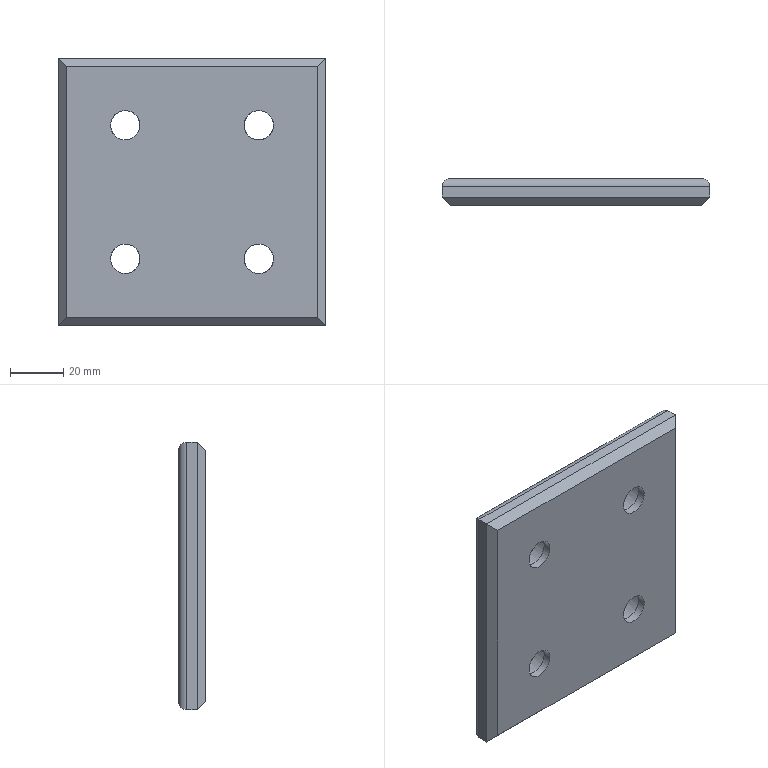Part | NX | features solid 2 | 1 solid | 26 faces | box 100 x 10 x 100 mm | volume 89599 mm3 | plane 14 | cylinder 12 | commonest cylinder face diameters 6 x4 11 x4 17.5 x4
STEP:
#1=CARTESIAN_POINT('',(-1385.,-327.,-360.));
#2=VERTEX_POINT('',#1);
#3=CARTESIAN_POINT('',(-1385.,-323.,-360.));
#4=VERTEX_POINT('',#3);
#5=CARTESIAN_POINT('',(-1385.,-330.,-360.));
#6=DIRECTION('',(0.,1.,0.));
#7=VECTOR('',#6,1000.);
#8=LINE('',#5,#7);
#9=EDGE_CURVE('',#2,#4,#8,.T.);
#10=ORIENTED_EDGE('',*,*,#9,.T.);
#11=CARTESIAN_POINT('',(-1385.,-323.,-260.));
#12=VERTEX_POINT('',#11);
#13=CARTESIAN_POINT('',(-1385.,-323.,-360.));
#14=DIRECTION('',(0.,0.,-1.));
#15=VECTOR('',#14,1000.);
#16=LINE('',#13,#15);
#17=EDGE_CURVE('',#12,#4,#16,.T.);
#18=ORIENTED_EDGE('',*,*,#17,.F.);
#19=CARTESIAN_POINT('',(-1385.,-327.,-260.));
#20=VERTEX_POINT('',#19);
#21=CARTESIAN_POINT('',(-1385.,-330.,-260.));
#22=DIRECTION('',(0.,1.,0.));
#23=VECTOR('',#22,1000.);
#24=LINE('',#21,#23);
#25=EDGE_CURVE('',#20,#12,#24,.T.);
#26=ORIENTED_EDGE('',*,*,#25,.F.);
#27=CARTESIAN_POINT('',(-1385.,-327.,-260.));
#28=DIRECTION('',(0.,0.,1.));
#29=VECTOR('',#28,1000.);
#30=LINE('',#27,#29);
#31=EDGE_CURVE('',#2,#20,#30,.T.);
#32=ORIENTED_EDGE('',*,*,#31,.F.);
#33=EDGE_LOOP('',(#10,#18,#26,#32));
#34=FACE_BOUND('',#33,.T.);
#35=CARTESIAN_POINT('',(-1385.,-330.,-260.));
#36=DIRECTION('',(-1.,0.,0.));
#37=DIRECTION('',(0.,0.,1.));
#38=AXIS2_PLACEMENT_3D('',#35,#36,#37);
#39=PLANE('',#38);
#40=ADVANCED_FACE('',(#34),#39,.F.);
#41=CARTESIAN_POINT('',(-1485.,-327.,-360.));
#42=VERTEX_POINT('',#41);
#43=CARTESIAN_POINT('',(-1485.,-323.,-360.));
#44=VERTEX_POINT('',#43);
#45=CARTESIAN_POINT('',(-1485.,-330.,-360.));
#46=DIRECTION('',(0.,1.,0.));
#47=VECTOR('',#46,1000.);
#48=LINE('',#45,#47);
#49=EDGE_CURVE('',#42,#44,#48,.T.);
#50=ORIENTED_EDGE('',*,*,#49,.T.);
#51=CARTESIAN_POINT('',(-1485.,-323.,-360.));
#52=DIRECTION('',(-1.,0.,0.));
#53=VECTOR('',#52,1000.);
#54=LINE('',#51,#53);
#55=EDGE_CURVE('',#4,#44,#54,.T.);
#56=ORIENTED_EDGE('',*,*,#55,.F.);
#57=ORIENTED_EDGE('',*,*,#9,.F.);
#58=CARTESIAN_POINT('',(-1385.,-327.,-360.));
#59=DIRECTION('',(1.,0.,0.));
#60=VECTOR('',#59,1000.);
#61=LINE('',#58,#60);
#62=EDGE_CURVE('',#42,#2,#61,.T.);
#63=ORIENTED_EDGE('',*,*,#62,.F.);
#64=EDGE_LOOP('',(#50,#56,#57,#63));
#65=FACE_BOUND('',#64,.T.);
#66=CARTESIAN_POINT('',(-1385.,-330.,-360.));
#67=DIRECTION('',(0.,0.,1.));
#68=DIRECTION('',(0.,-1.,0.));
#69=AXIS2_PLACEMENT_3D('',#66,#67,#68);
#70=PLANE('',#69);
#71=ADVANCED_FACE('',(#65),#70,.F.);
#72=CARTESIAN_POINT('',(-1485.,-327.,-260.));
#73=VERTEX_POINT('',#72);
#74=CARTESIAN_POINT('',(-1485.,-323.,-260.));
#75=VERTEX_POINT('',#74);
#76=CARTESIAN_POINT('',(-1485.,-330.,-260.));
#77=DIRECTION('',(0.,1.,0.));
#78=VECTOR('',#77,1000.);
#79=LINE('',#76,#78);
#80=EDGE_CURVE('',#73,#75,#79,.T.);
#81=ORIENTED_EDGE('',*,*,#80,.T.);
#82=CARTESIAN_POINT('',(-1485.,-323.,-260.));
#83=DIRECTION('',(0.,0.,1.));
#84=VECTOR('',#83,1000.);
#85=LINE('',#82,#84);
#86=EDGE_CURVE('',#44,#75,#85,.T.);
#87=ORIENTED_EDGE('',*,*,#86,.F.);
#88=ORIENTED_EDGE('',*,*,#49,.F.);
#89=CARTESIAN_POINT('',(-1485.,-327.,-360.));
#90=DIRECTION('',(0.,0.,-1.));
#91=VECTOR('',#90,1000.);
#92=LINE('',#89,#91);
#93=EDGE_CURVE('',#73,#42,#92,.T.);
#94=ORIENTED_EDGE('',*,*,#93,.F.);
#95=EDGE_LOOP('',(#81,#87,#88,#94));
#96=FACE_BOUND('',#95,.T.);
#97=CARTESIAN_POINT('',(-1485.,-330.,-360.));
#98=DIRECTION('',(1.,0.,0.));
#99=DIRECTION('',(0.,-1.,0.));
#100=AXIS2_PLACEMENT_3D('',#97,#98,#99);
#101=PLANE('',#100);
#102=ADVANCED_FACE('',(#96),#101,.F.);
#103=ORIENTED_EDGE('',*,*,#25,.T.);
#104=CARTESIAN_POINT('',(-1385.,-323.,-260.));
#105=DIRECTION('',(1.,0.,0.));
#106=VECTOR('',#105,1000.);
#107=LINE('',#104,#106);
#108=EDGE_CURVE('',#75,#12,#107,.T.);
#109=ORIENTED_EDGE('',*,*,#108,.F.);
#110=ORIENTED_EDGE('',*,*,#80,.F.);
#111=CARTESIAN_POINT('',(-1485.,-327.,-260.));
#112=DIRECTION('',(-1.,0.,0.));
#113=VECTOR('',#112,1000.);
#114=LINE('',#111,#113);
#115=EDGE_CURVE('',#20,#73,#114,.T.);
#116=ORIENTED_EDGE('',*,*,#115,.F.);
#117=EDGE_LOOP('',(#103,#109,#110,#116));
#118=FACE_BOUND('',#117,.T.);
#119=CARTESIAN_POINT('',(-1485.,-330.,-260.));
#120=DIRECTION('',(0.,0.,-1.));
#121=DIRECTION('',(-1.,0.,0.));
#122=AXIS2_PLACEMENT_3D('',#119,#120,#121);
#123=PLANE('',#122);
#124=ADVANCED_FACE('',(#118),#123,.F.);
#125=CARTESIAN_POINT('',(-1388.,-330.,-357.));
#126=VERTEX_POINT('',#125);
#127=CARTESIAN_POINT('',(-1482.,-330.,-357.));
#128=VERTEX_POINT('',#127);
#129=CARTESIAN_POINT('',(-1385.,-330.,-357.));
#130=DIRECTION('',(-1.,0.,0.));
#131=VECTOR('',#130,1000.);
#132=LINE('',#129,#131);
#133=EDGE_CURVE('',#126,#128,#132,.T.);
#134=ORIENTED_EDGE('',*,*,#133,.F.);
#135=CARTESIAN_POINT('',(-1388.,-330.,-263.));
#136=VERTEX_POINT('',#135);
#137=CARTESIAN_POINT('',(-1388.,-330.,-260.));
#138=DIRECTION('',(0.,0.,-1.));
#139=VECTOR('',#138,1000.);
#140=LINE('',#137,#139);
#141=EDGE_CURVE('',#136,#126,#140,.T.);
#142=ORIENTED_EDGE('',*,*,#141,.F.);
#143=CARTESIAN_POINT('',(-1482.,-330.,-263.));
#144=VERTEX_POINT('',#143);
#145=CARTESIAN_POINT('',(-1385.,-330.,-263.));
#146=DIRECTION('',(1.,0.,0.));
#147=VECTOR('',#146,1000.);
#148=LINE('',#145,#147);
#149=EDGE_CURVE('',#144,#136,#148,.T.);
#150=ORIENTED_EDGE('',*,*,#149,.F.);
#151=CARTESIAN_POINT('',(-1482.,-330.,-260.));
#152=DIRECTION('',(0.,0.,1.));
#153=VECTOR('',#152,1000.);
#154=LINE('',#151,#153);
#155=EDGE_CURVE('',#128,#144,#154,.T.);
#156=ORIENTED_EDGE('',*,*,#155,.F.);
#157=EDGE_LOOP('',(#134,#142,#150,#156));
#158=FACE_BOUND('',#157,.T.);
#159=CARTESIAN_POINT('',(-1454.5,-330.,-335.));
#160=VERTEX_POINT('',#159);
#161=CARTESIAN_POINT('',(-1460.,-330.,-335.));
#162=DIRECTION('',(0.,-1.,0.));
#163=DIRECTION('',(1.,0.,0.));
#164=AXIS2_PLACEMENT_3D('',#161,#162,#163);
#165=CIRCLE('',#164,5.5);
#166=EDGE_CURVE('',#160,#160,#165,.T.);
#167=ORIENTED_EDGE('',*,*,#166,.F.);
#168=EDGE_LOOP('',(#167));
#169=FACE_BOUND('',#168,.T.);
#170=CARTESIAN_POINT('',(-1454.5,-330.,-285.));
#171=VERTEX_POINT('',#170);
#172=CARTESIAN_POINT('',(-1460.,-330.,-285.));
#173=DIRECTION('',(0.,-1.,0.));
#174=DIRECTION('',(1.,0.,0.));
#175=AXIS2_PLACEMENT_3D('',#172,#173,#174);
#176=CIRCLE('',#175,5.5);
#177=EDGE_CURVE('',#171,#171,#176,.T.);
#178=ORIENTED_EDGE('',*,*,#177,.F.);
#179=EDGE_LOOP('',(#178));
#180=FACE_BOUND('',#179,.T.);
#181=CARTESIAN_POINT('',(-1404.5,-330.,-335.));
#182=VERTEX_POINT('',#181);
#183=CARTESIAN_POINT('',(-1410.,-330.,-335.));
#184=DIRECTION('',(0.,-1.,0.));
#185=DIRECTION('',(1.,0.,0.));
#186=AXIS2_PLACEMENT_3D('',#183,#184,#185);
#187=CIRCLE('',#186,5.5);
#188=EDGE_CURVE('',#182,#182,#187,.T.);
#189=ORIENTED_EDGE('',*,*,#188,.F.);
#190=EDGE_LOOP('',(#189));
#191=FACE_BOUND('',#190,.T.);
#192=CARTESIAN_POINT('',(-1404.5,-330.,-285.));
#193=VERTEX_POINT('',#192);
#194=CARTESIAN_POINT('',(-1410.,-330.,-285.));
#195=DIRECTION('',(0.,-1.,0.));
#196=DIRECTION('',(1.,0.,0.));
#197=AXIS2_PLACEMENT_3D('',#194,#195,#196);
#198=CIRCLE('',#197,5.5);
#199=EDGE_CURVE('',#193,#193,#198,.T.);
#200=ORIENTED_EDGE('',*,*,#199,.F.);
#201=EDGE_LOOP('',(#200));
#202=FACE_BOUND('',#201,.T.);
#203=CARTESIAN_POINT('',(-1385.,-330.,-260.));
#204=DIRECTION('',(0.,1.,0.));
#205=DIRECTION('',(1.,0.,0.));
#206=AXIS2_PLACEMENT_3D('',#203,#204,#205);
#207=PLANE('',#206);
#208=ADVANCED_FACE('',(#158,#169,#180,#191,#202),#207,.F.);
#209=CARTESIAN_POINT('',(-1388.,-320.,-357.));
#210=VERTEX_POINT('',#209);
#211=CARTESIAN_POINT('',(-1388.,-320.,-263.));
#212=VERTEX_POINT('',#211);
#213=CARTESIAN_POINT('',(-1388.,-320.,-260.));
#214=DIRECTION('',(0.,0.,-1.));
#215=VECTOR('',#214,1000.);
#216=LINE('',#213,#215);
#217=EDGE_CURVE('',#210,#212,#216,.F.);
#218=ORIENTED_EDGE('',*,*,#217,.F.);
#219=CARTESIAN_POINT('',(-1482.,-320.,-357.));
#220=VERTEX_POINT('',#219);
#221=CARTESIAN_POINT('',(-1385.,-320.,-357.));
#222=DIRECTION('',(-1.,0.,0.));
#223=VECTOR('',#222,1000.);
#224=LINE('',#221,#223);
#225=EDGE_CURVE('',#220,#210,#224,.F.);
#226=ORIENTED_EDGE('',*,*,#225,.F.);
#227=CARTESIAN_POINT('',(-1482.,-320.,-263.));
#228=VERTEX_POINT('',#227);
#229=CARTESIAN_POINT('',(-1482.,-320.,-360.));
#230=DIRECTION('',(0.,0.,1.));
#231=VECTOR('',#230,1000.);
#232=LINE('',#229,#231);
#233=EDGE_CURVE('',#228,#220,#232,.F.);
#234=ORIENTED_EDGE('',*,*,#233,.F.);
#235=CARTESIAN_POINT('',(-1485.,-320.,-263.));
#236=DIRECTION('',(1.,0.,0.));
#237=VECTOR('',#236,1000.);
#238=LINE('',#235,#237);
#239=EDGE_CURVE('',#212,#228,#238,.F.);
#240=ORIENTED_EDGE('',*,*,#239,.F.);
#241=EDGE_LOOP('',(#218,#226,#234,#240));
#242=FACE_BOUND('',#241,.T.);
#243=CARTESIAN_POINT('',(-1468.75,-320.,-335.));
#244=VERTEX_POINT('',#243);
#245=CARTESIAN_POINT('',(-1460.,-320.,-335.));
#246=DIRECTION('',(0.,1.,0.));
#247=DIRECTION('',(-1.,0.,0.));
#248=AXIS2_PLACEMENT_3D('',#245,#246,#247);
#249=CIRCLE('',#248,8.75);
#250=EDGE_CURVE('',#244,#244,#249,.T.);
#251=ORIENTED_EDGE('',*,*,#250,.F.);
#252=EDGE_LOOP('',(#251));
#253=FACE_BOUND('',#252,.T.);
#254=CARTESIAN_POINT('',(-1468.75,-320.,-285.));
#255=VERTEX_POINT('',#254);
#256=CARTESIAN_POINT('',(-1460.,-320.,-285.));
#257=DIRECTION('',(0.,1.,0.));
#258=DIRECTION('',(-1.,0.,0.));
#259=AXIS2_PLACEMENT_3D('',#256,#257,#258);
#260=CIRCLE('',#259,8.75);
#261=EDGE_CURVE('',#255,#255,#260,.T.);
#262=ORIENTED_EDGE('',*,*,#261,.F.);
#263=EDGE_LOOP('',(#262));
#264=FACE_BOUND('',#263,.T.);
#265=CARTESIAN_POINT('',(-1418.75,-320.,-335.));
#266=VERTEX_POINT('',#265);
#267=CARTESIAN_POINT('',(-1410.,-320.,-335.));
#268=DIRECTION('',(0.,1.,0.));
#269=DIRECTION('',(-1.,0.,0.));
#270=AXIS2_PLACEMENT_3D('',#267,#268,#269);
#271=CIRCLE('',#270,8.75);
#272=EDGE_CURVE('',#266,#266,#271,.T.);
#273=ORIENTED_EDGE('',*,*,#272,.F.);
#274=EDGE_LOOP('',(#273));
#275=FACE_BOUND('',#274,.T.);
#276=CARTESIAN_POINT('',(-1418.75,-320.,-285.));
#277=VERTEX_POINT('',#276);
#278=CARTESIAN_POINT('',(-1410.,-320.,-285.));
#279=DIRECTION('',(0.,1.,0.));
#280=DIRECTION('',(-1.,0.,0.));
#281=AXIS2_PLACEMENT_3D('',#278,#279,#280);
#282=CIRCLE('',#281,8.75);
#283=EDGE_CURVE('',#277,#277,#282,.T.);
#284=ORIENTED_EDGE('',*,*,#283,.F.);
#285=EDGE_LOOP('',(#284));
#286=FACE_BOUND('',#285,.T.);
#287=CARTESIAN_POINT('',(-1385.,-320.,-260.));
#288=DIRECTION('',(0.,1.,0.));
#289=DIRECTION('',(1.,0.,0.));
#290=AXIS2_PLACEMENT_3D('',#287,#288,#289);
#291=PLANE('',#290);
#292=ADVANCED_FACE('',(#242,#253,#264,#275,#286),#291,.T.);
#293=CARTESIAN_POINT('',(-1410.,-327.,-290.5));
#294=VERTEX_POINT('',#293);
#295=CARTESIAN_POINT('',(-1410.,-327.,-285.));
#296=DIRECTION('',(0.,1.,0.));
#297=DIRECTION('',(0.,0.,-1.));
#298=AXIS2_PLACEMENT_3D('',#295,#296,#297);
#299=CIRCLE('',#298,5.5);
#300=EDGE_CURVE('',#294,#294,#299,.T.);
#301=ORIENTED_EDGE('',*,*,#300,.T.);
#302=EDGE_LOOP('',(#301));
#303=FACE_BOUND('',#302,.T.);
#304=ORIENTED_EDGE('',*,*,#199,.T.);
#305=EDGE_LOOP('',(#304));
#306=FACE_BOUND('',#305,.T.);
#307=CARTESIAN_POINT('',(-1410.,-360.,-285.));
#308=DIRECTION('',(0.,-1.,0.));
#309=DIRECTION('',(-1.,0.,0.));
#310=AXIS2_PLACEMENT_3D('',#307,#308,#309);
#311=CYLINDRICAL_SURFACE('',#310,5.5);
#312=ADVANCED_FACE('',(#303,#306),#311,.F.);
#313=ORIENTED_EDGE('',*,*,#300,.F.);
#314=EDGE_LOOP('',(#313));
#315=FACE_BOUND('',#314,.T.);
#316=CARTESIAN_POINT('',(-1410.,-327.,-293.75));
#317=VERTEX_POINT('',#316);
#318=CARTESIAN_POINT('',(-1410.,-327.,-285.));
#319=DIRECTION('',(0.,1.,0.));
#320=DIRECTION('',(0.,0.,-1.));
#321=AXIS2_PLACEMENT_3D('',#318,#319,#320);
#322=CIRCLE('',#321,8.75);
#323=EDGE_CURVE('',#317,#317,#322,.T.);
#324=ORIENTED_EDGE('',*,*,#323,.T.);
#325=EDGE_LOOP('',(#324));
#326=FACE_BOUND('',#325,.T.);
#327=CARTESIAN_POINT('',(-1410.,-327.,-285.));
#328=DIRECTION('',(0.,-1.,0.));
#329=DIRECTION('',(-1.,0.,0.));
#330=AXIS2_PLACEMENT_3D('',#327,#328,#329);
#331=PLANE('',#330);
#332=ADVANCED_FACE('',(#315,#326),#331,.F.);
#333=ORIENTED_EDGE('',*,*,#323,.F.);
#334=EDGE_LOOP('',(#333));
#335=FACE_BOUND('',#334,.T.);
#336=ORIENTED_EDGE('',*,*,#283,.T.);
#337=EDGE_LOOP('',(#336));
#338=FACE_BOUND('',#337,.T.);
#339=CARTESIAN_POINT('',(-1410.,-310.,-285.));
#340=DIRECTION('',(0.,-1.,0.));
#341=DIRECTION('',(-1.,0.,0.));
#342=AXIS2_PLACEMENT_3D('',#339,#340,#341);
#343=CYLINDRICAL_SURFACE('',#342,8.75);
#344=ADVANCED_FACE('',(#335,#338),#343,.F.);
#345=CARTESIAN_POINT('',(-1410.,-327.,-340.5));
#346=VERTEX_POINT('',#345);
#347=CARTESIAN_POINT('',(-1410.,-327.,-335.));
#348=DIRECTION('',(0.,1.,0.));
#349=DIRECTION('',(0.,0.,-1.));
#350=AXIS2_PLACEMENT_3D('',#347,#348,#349);
#351=CIRCLE('',#350,5.5);
#352=EDGE_CURVE('',#346,#346,#351,.T.);
#353=ORIENTED_EDGE('',*,*,#352,.T.);
#354=EDGE_LOOP('',(#353));
#355=FACE_BOUND('',#354,.T.);
#356=ORIENTED_EDGE('',*,*,#188,.T.);
#357=EDGE_LOOP('',(#356));
#358=FACE_BOUND('',#357,.T.);
#359=CARTESIAN_POINT('',(-1410.,-360.,-335.));
#360=DIRECTION('',(0.,-1.,0.));
#361=DIRECTION('',(-1.,0.,0.));
#362=AXIS2_PLACEMENT_3D('',#359,#360,#361);
#363=CYLINDRICAL_SURFACE('',#362,5.5);
#364=ADVANCED_FACE('',(#355,#358),#363,.F.);
#365=ORIENTED_EDGE('',*,*,#352,.F.);
#366=EDGE_LOOP('',(#365));
#367=FACE_BOUND('',#366,.T.);
#368=CARTESIAN_POINT('',(-1410.,-327.,-343.75));
#369=VERTEX_POINT('',#368);
#370=CARTESIAN_POINT('',(-1410.,-327.,-335.));
#371=DIRECTION('',(0.,1.,0.));
#372=DIRECTION('',(0.,0.,-1.));
#373=AXIS2_PLACEMENT_3D('',#370,#371,#372);
#374=CIRCLE('',#373,8.75);
#375=EDGE_CURVE('',#369,#369,#374,.T.);
#376=ORIENTED_EDGE('',*,*,#375,.T.);
#377=EDGE_LOOP('',(#376));
#378=FACE_BOUND('',#377,.T.);
#379=CARTESIAN_POINT('',(-1410.,-327.,-335.));
#380=DIRECTION('',(0.,-1.,0.));
#381=DIRECTION('',(-1.,0.,0.));
#382=AXIS2_PLACEMENT_3D('',#379,#380,#381);
#383=PLANE('',#382);
#384=ADVANCED_FACE('',(#367,#378),#383,.F.);
#385=ORIENTED_EDGE('',*,*,#375,.F.);
#386=EDGE_LOOP('',(#385));
#387=FACE_BOUND('',#386,.T.);
#388=ORIENTED_EDGE('',*,*,#272,.T.);
#389=EDGE_LOOP('',(#388));
#390=FACE_BOUND('',#389,.T.);
#391=CARTESIAN_POINT('',(-1410.,-310.,-335.));
#392=DIRECTION('',(0.,-1.,0.));
#393=DIRECTION('',(-1.,0.,0.));
#394=AXIS2_PLACEMENT_3D('',#391,#392,#393);
#395=CYLINDRICAL_SURFACE('',#394,8.75);
#396=ADVANCED_FACE('',(#387,#390),#395,.F.);
#397=CARTESIAN_POINT('',(-1460.,-327.,-290.5));
#398=VERTEX_POINT('',#397);
#399=CARTESIAN_POINT('',(-1460.,-327.,-285.));
#400=DIRECTION('',(0.,1.,0.));
#401=DIRECTION('',(0.,0.,-1.));
#402=AXIS2_PLACEMENT_3D('',#399,#400,#401);
#403=CIRCLE('',#402,5.5);
#404=EDGE_CURVE('',#398,#398,#403,.T.);
#405=ORIENTED_EDGE('',*,*,#404,.T.);
#406=EDGE_LOOP('',(#405));
#407=FACE_BOUND('',#406,.T.);
#408=ORIENTED_EDGE('',*,*,#177,.T.);
#409=EDGE_LOOP('',(#408));
#410=FACE_BOUND('',#409,.T.);
#411=CARTESIAN_POINT('',(-1460.,-360.,-285.));
#412=DIRECTION('',(0.,-1.,0.));
#413=DIRECTION('',(-1.,0.,0.));
#414=AXIS2_PLACEMENT_3D('',#411,#412,#413);
#415=CYLINDRICAL_SURFACE('',#414,5.5);
#416=ADVANCED_FACE('',(#407,#410),#415,.F.);
#417=ORIENTED_EDGE('',*,*,#404,.F.);
#418=EDGE_LOOP('',(#417));
#419=FACE_BOUND('',#418,.T.);
#420=CARTESIAN_POINT('',(-1460.,-327.,-293.75));
#421=VERTEX_POINT('',#420);
#422=CARTESIAN_POINT('',(-1460.,-327.,-285.));
#423=DIRECTION('',(0.,1.,0.));
#424=DIRECTION('',(0.,0.,-1.));
#425=AXIS2_PLACEMENT_3D('',#422,#423,#424);
#426=CIRCLE('',#425,8.75);
#427=EDGE_CURVE('',#421,#421,#426,.T.);
#428=ORIENTED_EDGE('',*,*,#427,.T.);
#429=EDGE_LOOP('',(#428));
#430=FACE_BOUND('',#429,.T.);
#431=CARTESIAN_POINT('',(-1460.,-327.,-285.));
#432=DIRECTION('',(0.,-1.,0.));
#433=DIRECTION('',(-1.,0.,0.));
#434=AXIS2_PLACEMENT_3D('',#431,#432,#433);
#435=PLANE('',#434);
#436=ADVANCED_FACE('',(#419,#430),#435,.F.);
#437=ORIENTED_EDGE('',*,*,#427,.F.);
#438=EDGE_LOOP('',(#437));
#439=FACE_BOUND('',#438,.T.);
#440=ORIENTED_EDGE('',*,*,#261,.T.);
#441=EDGE_LOOP('',(#440));
#442=FACE_BOUND('',#441,.T.);
#443=CARTESIAN_POINT('',(-1460.,-310.,-285.));
#444=DIRECTION('',(0.,-1.,0.));
#445=DIRECTION('',(-1.,0.,0.));
#446=AXIS2_PLACEMENT_3D('',#443,#444,#445);
#447=CYLINDRICAL_SURFACE('',#446,8.75);
#448=ADVANCED_FACE('',(#439,#442),#447,.F.);
#449=CARTESIAN_POINT('',(-1460.,-327.,-340.5));
#450=VERTEX_POINT('',#449);
#451=CARTESIAN_POINT('',(-1460.,-327.,-335.));
#452=DIRECTION('',(0.,1.,0.));
#453=DIRECTION('',(0.,0.,-1.));
#454=AXIS2_PLACEMENT_3D('',#451,#452,#453);
#455=CIRCLE('',#454,5.5);
#456=EDGE_CURVE('',#450,#450,#455,.T.);
#457=ORIENTED_EDGE('',*,*,#456,.T.);
#458=EDGE_LOOP('',(#457));
#459=FACE_BOUND('',#458,.T.);
#460=ORIENTED_EDGE('',*,*,#166,.T.);
#461=EDGE_LOOP('',(#460));
#462=FACE_BOUND('',#461,.T.);
#463=CARTESIAN_POINT('',(-1460.,-360.,-335.));
#464=DIRECTION('',(0.,-1.,0.));
#465=DIRECTION('',(-1.,0.,0.));
#466=AXIS2_PLACEMENT_3D('',#463,#464,#465);
#467=CYLINDRICAL_SURFACE('',#466,5.5);
#468=ADVANCED_FACE('',(#459,#462),#467,.F.);
#469=ORIENTED_EDGE('',*,*,#456,.F.);
#470=EDGE_LOOP('',(#469));
#471=FACE_BOUND('',#470,.T.);
#472=CARTESIAN_POINT('',(-1460.,-327.,-343.75));
#473=VERTEX_POINT('',#472);
#474=CARTESIAN_POINT('',(-1460.,-327.,-335.));
#475=DIRECTION('',(0.,1.,0.));
#476=DIRECTION('',(0.,0.,-1.));
#477=AXIS2_PLACEMENT_3D('',#474,#475,#476);
#478=CIRCLE('',#477,8.75);
#479=EDGE_CURVE('',#473,#473,#478,.T.);
#480=ORIENTED_EDGE('',*,*,#479,.T.);
#481=EDGE_LOOP('',(#480));
#482=FACE_BOUND('',#481,.T.);
#483=CARTESIAN_POINT('',(-1460.,-327.,-335.));
#484=DIRECTION('',(0.,-1.,0.));
#485=DIRECTION('',(-1.,0.,0.));
#486=AXIS2_PLACEMENT_3D('',#483,#484,#485);
#487=PLANE('',#486);
#488=ADVANCED_FACE('',(#471,#482),#487,.F.);
#489=ORIENTED_EDGE('',*,*,#479,.F.);
#490=EDGE_LOOP('',(#489));
#491=FACE_BOUND('',#490,.T.);
#492=ORIENTED_EDGE('',*,*,#250,.T.);
#493=EDGE_LOOP('',(#492));
#494=FACE_BOUND('',#493,.T.);
#495=CARTESIAN_POINT('',(-1460.,-310.,-335.));
#496=DIRECTION('',(0.,-1.,0.));
#497=DIRECTION('',(-1.,0.,0.));
#498=AXIS2_PLACEMENT_3D('',#495,#496,#497);
#499=CYLINDRICAL_SURFACE('',#498,8.75);
#500=ADVANCED_FACE('',(#491,#494),#499,.F.);
#501=CARTESIAN_POINT('',(-1388.,-323.,-357.));
#502=DIRECTION('',(-0.7071,0.,-0.7071));
#503=DIRECTION('',(-0.7071,0.,0.7071));
#504=AXIS2_PLACEMENT_3D('',#501,#502,#503);
#505=ELLIPSE('',#504,4.243,3.);
#506=EDGE_CURVE('',#210,#4,#505,.T.);
#507=ORIENTED_EDGE('',*,*,#506,.T.);
#508=ORIENTED_EDGE('',*,*,#55,.T.);
#509=CARTESIAN_POINT('',(-1482.,-323.,-357.));
#510=DIRECTION('',(-0.7071,0.,0.7071));
#511=DIRECTION('',(0.7071,0.,0.7071));
#512=AXIS2_PLACEMENT_3D('',#509,#510,#511);
#513=ELLIPSE('',#512,4.243,3.);
#514=EDGE_CURVE('',#44,#220,#513,.F.);
#515=ORIENTED_EDGE('',*,*,#514,.T.);
#516=ORIENTED_EDGE('',*,*,#225,.T.);
#517=EDGE_LOOP('',(#507,#508,#515,#516));
#518=FACE_BOUND('',#517,.T.);
#519=CARTESIAN_POINT('',(-1385.,-323.,-357.));
#520=DIRECTION('',(1.,0.,0.));
#521=DIRECTION('',(0.,-1.,0.));
#522=AXIS2_PLACEMENT_3D('',#519,#520,#521);
#523=CYLINDRICAL_SURFACE('',#522,3.);
#524=ADVANCED_FACE('',(#518),#523,.T.);
#525=ORIENTED_EDGE('',*,*,#514,.F.);
#526=ORIENTED_EDGE('',*,*,#86,.T.);
#527=CARTESIAN_POINT('',(-1482.,-323.,-263.));
#528=DIRECTION('',(0.7071,0.,0.7071));
#529=DIRECTION('',(0.7071,0.,-0.7071));
#530=AXIS2_PLACEMENT_3D('',#527,#528,#529);
#531=ELLIPSE('',#530,4.243,3.);
#532=EDGE_CURVE('',#75,#228,#531,.F.);
#533=ORIENTED_EDGE('',*,*,#532,.T.);
#534=ORIENTED_EDGE('',*,*,#233,.T.);
#535=EDGE_LOOP('',(#525,#526,#533,#534));
#536=FACE_BOUND('',#535,.T.);
#537=CARTESIAN_POINT('',(-1482.,-323.,-360.));
#538=DIRECTION('',(0.,0.,-1.));
#539=DIRECTION('',(0.,1.,0.));
#540=AXIS2_PLACEMENT_3D('',#537,#538,#539);
#541=CYLINDRICAL_SURFACE('',#540,3.);
#542=ADVANCED_FACE('',(#536),#541,.T.);
#543=ORIENTED_EDGE('',*,*,#506,.F.);
#544=ORIENTED_EDGE('',*,*,#217,.T.);
#545=CARTESIAN_POINT('',(-1388.,-323.,-263.));
#546=DIRECTION('',(0.7071,0.,-0.7071));
#547=DIRECTION('',(0.7071,0.,0.7071));
#548=AXIS2_PLACEMENT_3D('',#545,#546,#547);
#549=ELLIPSE('',#548,4.243,3.);
#550=EDGE_CURVE('',#212,#12,#549,.T.);
#551=ORIENTED_EDGE('',*,*,#550,.T.);
#552=ORIENTED_EDGE('',*,*,#17,.T.);
#553=EDGE_LOOP('',(#543,#544,#551,#552));
#554=FACE_BOUND('',#553,.T.);
#555=CARTESIAN_POINT('',(-1388.,-323.,-260.));
#556=DIRECTION('',(0.,0.,1.));
#557=DIRECTION('',(1.,0.,0.));
#558=AXIS2_PLACEMENT_3D('',#555,#556,#557);
#559=CYLINDRICAL_SURFACE('',#558,3.);
#560=ADVANCED_FACE('',(#554),#559,.T.);
#561=ORIENTED_EDGE('',*,*,#532,.F.);
#562=ORIENTED_EDGE('',*,*,#108,.T.);
#563=ORIENTED_EDGE('',*,*,#550,.F.);
#564=ORIENTED_EDGE('',*,*,#239,.T.);
#565=EDGE_LOOP('',(#561,#562,#563,#564));
#566=FACE_BOUND('',#565,.T.);
#567=CARTESIAN_POINT('',(-1485.,-323.,-263.));
#568=DIRECTION('',(-1.,0.,0.));
#569=DIRECTION('',(0.,0.,1.));
#570=AXIS2_PLACEMENT_3D('',#567,#568,#569);
#571=CYLINDRICAL_SURFACE('',#570,3.);
#572=ADVANCED_FACE('',(#566),#571,.T.);
#573=CARTESIAN_POINT('',(-1387.,-329.,-262.));
#574=DIRECTION('',(-0.5774,-0.5774,-0.5774));
#575=VECTOR('',#574,1000.);
#576=LINE('',#573,#575);
#577=EDGE_CURVE('',#20,#136,#576,.T.);
#578=ORIENTED_EDGE('',*,*,#577,.T.);
#579=ORIENTED_EDGE('',*,*,#141,.T.);
#580=CARTESIAN_POINT('',(-1420.333,-362.333,-324.667));
#581=DIRECTION('',(-0.5774,-0.5774,0.5774));
#582=VECTOR('',#581,1000.);
#583=LINE('',#580,#582);
#584=EDGE_CURVE('',#126,#2,#583,.F.);
#585=ORIENTED_EDGE('',*,*,#584,.T.);
#586=ORIENTED_EDGE('',*,*,#31,.T.);
#587=EDGE_LOOP('',(#578,#579,#585,#586));
#588=FACE_BOUND('',#587,.T.);
#589=CARTESIAN_POINT('',(-1388.,-330.,-260.));
#590=DIRECTION('',(-0.7071,0.7071,0.));
#591=DIRECTION('',(0.7071,0.7071,0.));
#592=AXIS2_PLACEMENT_3D('',#589,#590,#591);
#593=PLANE('',#592);
#594=ADVANCED_FACE('',(#588),#593,.F.);
#595=ORIENTED_EDGE('',*,*,#584,.F.);
#596=ORIENTED_EDGE('',*,*,#133,.T.);
#597=CARTESIAN_POINT('',(-1449.667,-362.333,-324.667));
#598=DIRECTION('',(0.5774,-0.5774,0.5774));
#599=VECTOR('',#598,1000.);
#600=LINE('',#597,#599);
#601=EDGE_CURVE('',#128,#42,#600,.F.);
#602=ORIENTED_EDGE('',*,*,#601,.T.);
#603=ORIENTED_EDGE('',*,*,#62,.T.);
#604=EDGE_LOOP('',(#595,#596,#602,#603));
#605=FACE_BOUND('',#604,.T.);
#606=CARTESIAN_POINT('',(-1385.,-330.,-357.));
#607=DIRECTION('',(0.,0.7071,0.7071));
#608=DIRECTION('',(0.,-0.7071,0.7071));
#609=AXIS2_PLACEMENT_3D('',#606,#607,#608);
#610=PLANE('',#609);
#611=ADVANCED_FACE('',(#605),#610,.F.);
#612=ORIENTED_EDGE('',*,*,#577,.F.);
#613=ORIENTED_EDGE('',*,*,#115,.T.);
#614=CARTESIAN_POINT('',(-1449.667,-362.333,-295.333));
#615=DIRECTION('',(-0.5774,0.5774,0.5774));
#616=VECTOR('',#615,1000.);
#617=LINE('',#614,#616);
#618=EDGE_CURVE('',#73,#144,#617,.F.);
#619=ORIENTED_EDGE('',*,*,#618,.T.);
#620=ORIENTED_EDGE('',*,*,#149,.T.);
#621=EDGE_LOOP('',(#612,#613,#619,#620));
#622=FACE_BOUND('',#621,.T.);
#623=CARTESIAN_POINT('',(-1385.,-330.,-263.));
#624=DIRECTION('',(0.,0.7071,-0.7071));
#625=DIRECTION('',(0.,0.7071,0.7071));
#626=AXIS2_PLACEMENT_3D('',#623,#624,#625);
#627=PLANE('',#626);
#628=ADVANCED_FACE('',(#622),#627,.F.);
#629=ORIENTED_EDGE('',*,*,#601,.F.);
#630=ORIENTED_EDGE('',*,*,#155,.T.);
#631=ORIENTED_EDGE('',*,*,#618,.F.);
#632=ORIENTED_EDGE('',*,*,#93,.T.);
#633=EDGE_LOOP('',(#629,#630,#631,#632));
#634=FACE_BOUND('',#633,.T.);
#635=CARTESIAN_POINT('',(-1482.,-330.,-260.));
#636=DIRECTION('',(0.7071,0.7071,0.));
#637=DIRECTION('',(0.7071,-0.7071,0.));
#638=AXIS2_PLACEMENT_3D('',#635,#636,#637);
#639=PLANE('',#638);
#640=ADVANCED_FACE('',(#634),#639,.F.);
#641=CLOSED_SHELL('',(#40,#71,#102,#124,#208,#292,#312,#332,#344,#364,#384,#396,#416,#436,#448,#468,#488,#500,#524,#542,#560,#572,#594,#611,#628,#640));
#642=MANIFOLD_SOLID_BREP('',#641);
#643=(LENGTH_UNIT()NAMED_UNIT(*)SI_UNIT(.MILLI.,.METRE.));
#644=UNCERTAINTY_MEASURE_WITH_UNIT(LENGTH_MEASURE(0.00001),#643,'','');
#645=(NAMED_UNIT(*)PLANE_ANGLE_UNIT()SI_UNIT($,.RADIAN.));
#646=(NAMED_UNIT(*)SI_UNIT($,.STERADIAN.)SOLID_ANGLE_UNIT());
#647=(GEOMETRIC_REPRESENTATION_CONTEXT(3)GLOBAL_UNCERTAINTY_ASSIGNED_CONTEXT((#644))GLOBAL_UNIT_ASSIGNED_CONTEXT((#643,#645,#646))REPRESENTATION_CONTEXT('',''));
#648=ADVANCED_BREP_SHAPE_REPRESENTATION('',(#642),#647);